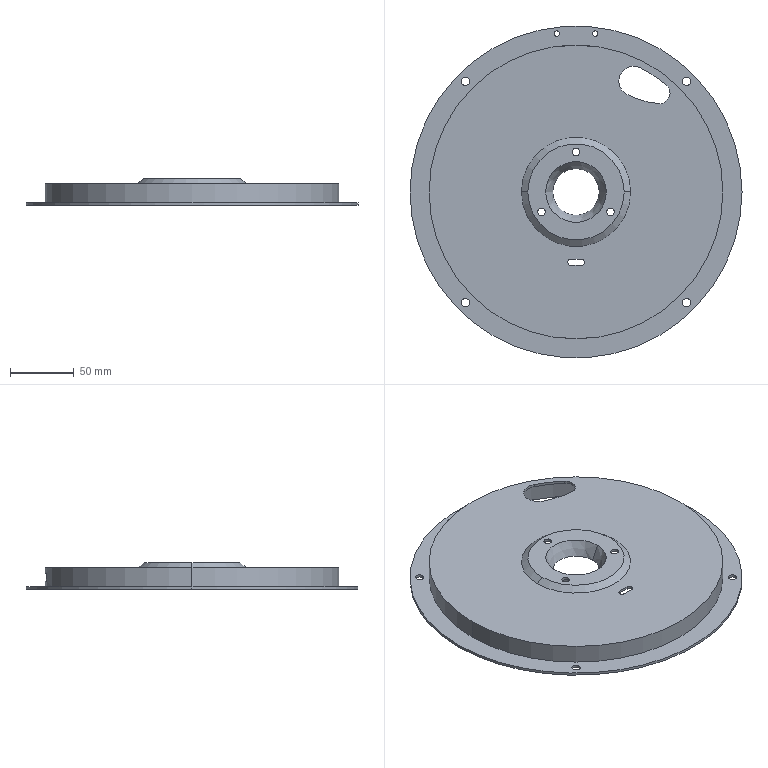Part | SolidWorks | features ICE 5, CirPattern 2, 3DProfileFeature 1, HoleWzd 1, Revolution 1 | 1 solid | 56 faces | box 260 x 260 x 21 mm | volume 125361 mm3 | cylinder 29 | cone 14 | plane 13 | commonest cylinder face diameters 6.5 x8 6 x6 5 x3 23.455 x2 226 x2 230 x2